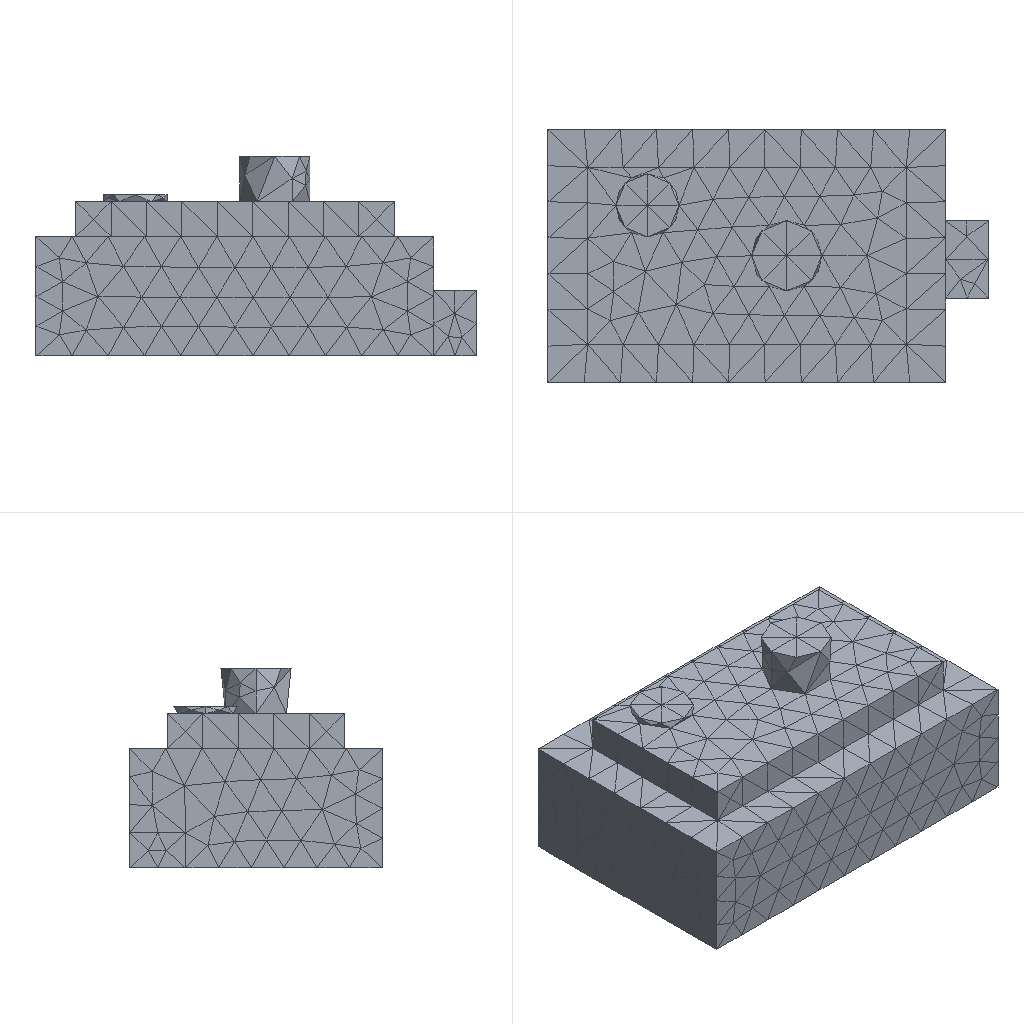Simulation study | ansys mapdl
Set-up summary:
category,name,step,type,value,unit,region
solver,ansys_mapdl
units,mm-N-s-tonne (MPa),,inferred,E=210000 density=
analysis,model,,static
mesh,nodes,,,4626
mesh,elements,,,2765
element_type,SOLID187,,,2765
material,mat 1,,E,210000
material,mat 1,,nu,0.3
load,,model,body load temp,,,all
load,,model,force,"1000 [dir=(0, 0, -1) n=128]",,node list
bc,,model,fixed,"[dofs=UX,UY,UZ n=5081]",,node list
Ansys APDL input file, long lists of numbers shortened:
/COM,ANSYS RELEASE 2026 R1           BUILD 26.1      UP20260202       09:09:22
/PREP7
/NOPR
/TITLE,2
ANTYPE, 0
*IF,_CDRDOFF,EQ,1,THEN     !if solid model was read in
_CDRDOFF=             !reset flag, numoffs already performed
*ELSE              !offset database for the following FE model
NUMOFF,NODE,     4626
NUMOFF,ELEM,     2765
NUMOFF,MAT ,        1
NUMOFF,TYPE,        1
*ENDIF
*SET,_RETURN ,  0.
*SET,_STATUS ,  0.
*SET,_UIQR   ,  128.
*SET,__FLOATPARAMETER__,  4626.
DOF,DELETE
ETBLOCK,        1,        1
(2i9,19a9)
        1      187        0        0        0        0        0        0        0        0        0        0        0        0        0        0        0        0        0        0        0
       -1
NBLOCK,6,SOLID,      4626,      4626
(3i9,6e21.13e3)
        1        0        0-4.0725000000000E+001 3.6000000000000E+001 1.0000000000000E+001
! (4625 more lines like these left out)
N,UNBL,LOC,       -1,
EBLOCK,19,SOLID,      2765,      2765
(19i10)
         1         1         1         1         0         0         0         0        10         0         1      1771      1772      1773      1774      2037      2038      2039      2040
! (5529 more lines like these left out)
        -1
MPTEMP,UNBL, 1, 1,  0.    ,
MPDATA,UNBL, 1,EX  ,       1, 1,  210000.000    ,
MPTEMP,UNBL, 1, 1,  0.    ,
MPDATA,UNBL, 1,NUXY,       1, 1, 0.3    ,
MPTEMP,UNBL, 1, 1,  0.    ,
MPDATA,UNBL, 1,PRXY,       1, 1, 0.3    ,
EXTOPT,ATTR,      0,      0,      0
EXTOPT,ESIZE,  0,  0.
EXTOPT,ACLEAR,      0
TREF,  0.
IRLF,  0
BFUNIF,TEMP,_TINY
ACEL,  0.    ,  0.    ,  0.
OMEGA,  0.    ,  0.    ,  0.
DOMEGA,  0.    ,  0.    ,  0.
CGLOC,  0.    ,  0.    ,  0.
CGOMEGA,  0.    ,  0.    ,  0.
DCGOMG,  0.    ,  0.    ,  0.
KUSE,     0
TIME,  0.
ALPHAD,  0.
BETAD,  0.
DMPRAT,  0.
DMPSTR,  0.
CRPLIM, 0.1    ,   0
CRPLIM,  0.    ,   1
NCNV,     0, 1.000000000E+12,     0,  0.    ,  0.
NEQIT,     0
ERESX,DEFA
DBLOCK,      5081
(i9,a6,2(pg16.9))
        1  UX    0.00000000      0.00000000
! (5080 more lines like these left out)
       -1
FBLOCK,       128
(i9,a6,2(pg16.9))
      923  FZ   -7.81250000      0.00000000
! (127 more lines like these left out)
       -1
/GO
FINISH
Results summary:
result,analysis_type_db,,,static,unstated
result,n_sets,,,1,unstated
result,load_steps[0].set,load_step=1,,1,unstated
result,load_steps[0].substep,load_step=1,,1,unstated
result,load_steps[0].time,load_step=1,,1,unstated
result,load_steps[0].freq,load_step=1,,1,unstated
result,load_steps[0].max_usum,load_step=1,,0.0003393,unstated
result,load_steps[0].max_seqv,load_step=1,,4.428,unstated
result,load_steps[0].reaction_sum.FX,load_step=1,,2.23821e-12,unstated
result,load_steps[0].reaction_sum.FY,load_step=1,,-4.19575e-12,unstated
result,load_steps[0].reaction_sum.FZ,load_step=1,,1000,unstated
result,load_steps[0].reaction_sum.MX,load_step=1,,0,unstated
result,load_steps[0].reaction_sum.MY,load_step=1,,0,unstated
result,load_steps[0].reaction_sum.MZ,load_step=1,,0,unstated
result,convergence,,,results present for all listed sets,unstated